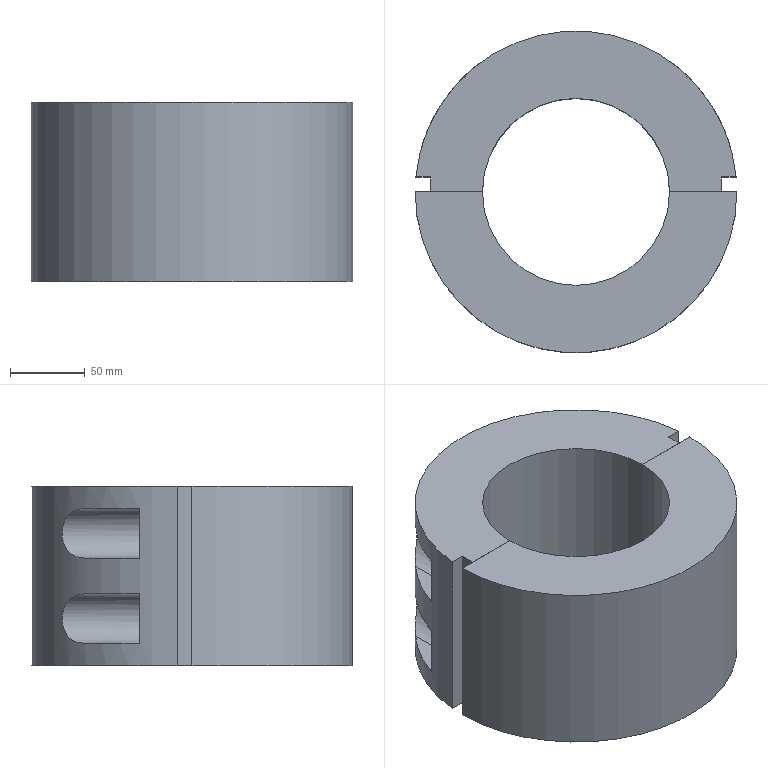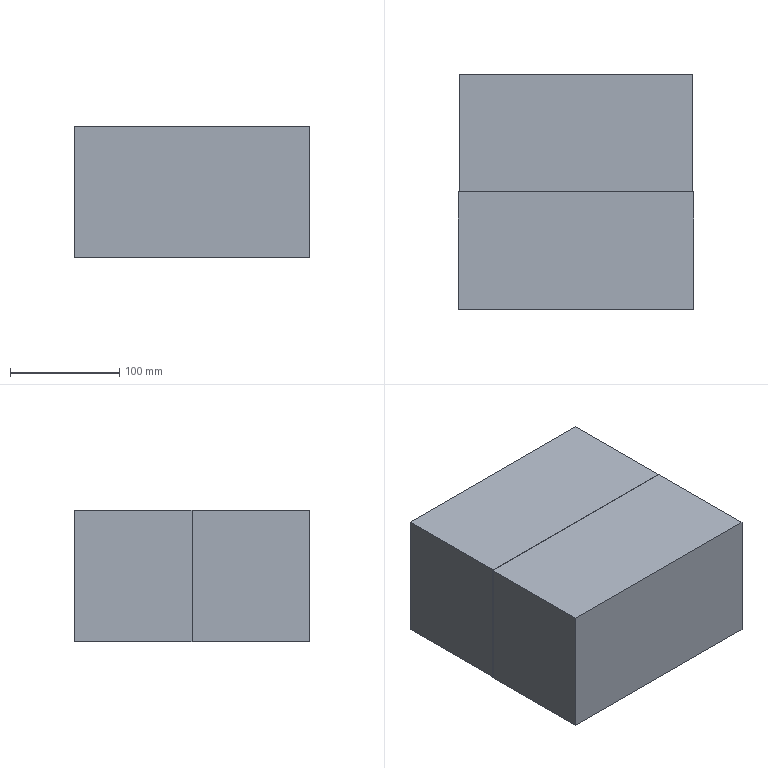CAM job | NX | 3-axis milling, drilling | part box 215 x 215 x 120 mm | stock box 215 x 215 x 120 mm
Tools:
number,name,description,diameter,corner_radius,flute_length,length,flutes
1,D25,Milling Tool-5 Parameters,25.0,0.0,50.0,75.0,2
2,ZXZ,Milling Tool-5 Parameters,6.0,0.0,50.0,75.0,2
3,21.5ZT,Drilling Tool,21.5,0.0,35.0,50.0,2
4,17.5ZT,Drilling Tool,17.5,0.0,35.0,50.0,2
5,D15XYD,Thread Mill,15.0,0.0,2.5,50.0,2
Operations:
program,operation,operation_type,tool,method,geometry_group,spindle_rpm,surface_speed,feed_per_tooth,feed_cut,feed_plunge,cut_length_mm,path_length_mm,cut_time_min,machine_time_min
215-125-120,ZLEVEL_PROFILE,ZLevelMilling,D25,METHOD,A,1000.0,78.0,1.0,2000.0,100.0,34904.088,36160.149,17.452,17.578
215-125-120,DRILLING,Operation,ZXZ,METHOD,A,3500.0,65.0,0.0357,250.0,0.0,16.0,520.186,0.064,0.1144
215-125-120,DRILLING_COPY,Operation,21.5ZT,METHOD,A,500.0,33.0,0.08,80.0,0.0,183.837,855.86,2.298,2.365
XY215-125-120,DRILLING_COPY_1,Operation,ZXZ,METHOD,B,3500.0,65.0,0.0357,250.0,0.0,16.0,375.186,0.064,0.0999
XY215-125-120,DRILLING_COPY_COPY,Operation,17.5ZT,METHOD,B,500.0,33.0,0.08,80.0,0.0,173.03,689.246,2.163,2.215
XY215-125-120,THREAD_MILLING,ThreadMilling,D15XYD,METHOD,B,1200.0,56.0,0.2083,500.0,100.0,2421.239,3305.23,4.843,4.931